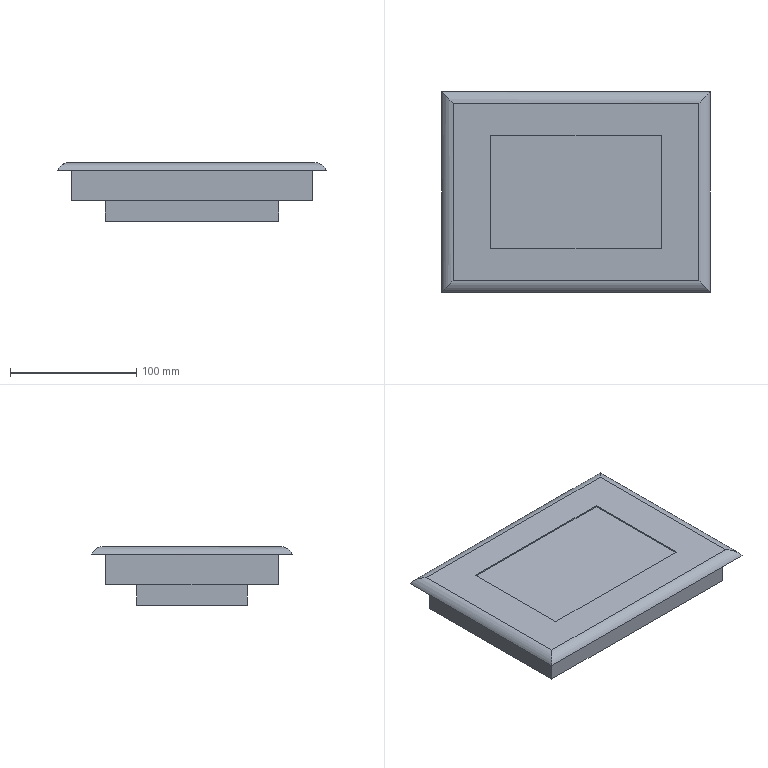Part | STEP file | 7-inch Weintek touch screen TH765-N[7-inch Weintek touch screen TH765-N]_7-inch Weintek touch screen TH765-N | 1 solid | 21 faces | box 213 x 159 x 46.5 mm | volume 1006657 mm3 | plane 17 | cylinder 4 | commonest cylinder face diameters 20 x4
STEP:
#1=CARTESIAN_POINT('',(97.335,-70.335,6.));
#2=VERTEX_POINT('',#1);
#3=CARTESIAN_POINT('',(-97.335,-70.335,6.));
#4=VERTEX_POINT('',#3);
#5=CARTESIAN_POINT('',(0.,-70.335,6.));
#6=DIRECTION('',(-1.,0.,0.));
#7=VECTOR('',#6,1000.);
#8=LINE('',#5,#7);
#9=EDGE_CURVE('',#2,#4,#8,.T.);
#10=ORIENTED_EDGE('',*,*,#9,.F.);
#11=CARTESIAN_POINT('',(97.335,70.335,6.));
#12=VERTEX_POINT('',#11);
#13=CARTESIAN_POINT('',(97.335,0.,6.));
#14=DIRECTION('',(0.,-1.,0.));
#15=VECTOR('',#14,1000.);
#16=LINE('',#13,#15);
#17=EDGE_CURVE('',#12,#2,#16,.T.);
#18=ORIENTED_EDGE('',*,*,#17,.F.);
#19=CARTESIAN_POINT('',(-97.335,70.335,6.));
#20=VERTEX_POINT('',#19);
#21=CARTESIAN_POINT('',(0.,70.335,6.));
#22=DIRECTION('',(1.,0.,0.));
#23=VECTOR('',#22,1000.);
#24=LINE('',#21,#23);
#25=EDGE_CURVE('',#20,#12,#24,.T.);
#26=ORIENTED_EDGE('',*,*,#25,.F.);
#27=CARTESIAN_POINT('',(-97.335,0.,6.));
#28=DIRECTION('',(0.,1.,0.));
#29=VECTOR('',#28,1000.);
#30=LINE('',#27,#29);
#31=EDGE_CURVE('',#4,#20,#30,.T.);
#32=ORIENTED_EDGE('',*,*,#31,.F.);
#33=EDGE_LOOP('',(#10,#18,#26,#32));
#34=FACE_OUTER_BOUND('',#33,.T.);
#35=CARTESIAN_POINT('',(67.5,-45.,6.));
#36=VERTEX_POINT('',#35);
#37=CARTESIAN_POINT('',(67.5,45.,6.));
#38=VERTEX_POINT('',#37);
#39=CARTESIAN_POINT('',(67.5,0.,6.));
#40=DIRECTION('',(0.,1.,0.));
#41=VECTOR('',#40,1000.);
#42=LINE('',#39,#41);
#43=EDGE_CURVE('',#36,#38,#42,.T.);
#44=ORIENTED_EDGE('',*,*,#43,.F.);
#45=CARTESIAN_POINT('',(-67.5,-45.,6.));
#46=VERTEX_POINT('',#45);
#47=CARTESIAN_POINT('',(0.,-45.,6.));
#48=DIRECTION('',(1.,0.,0.));
#49=VECTOR('',#48,1000.);
#50=LINE('',#47,#49);
#51=EDGE_CURVE('',#46,#36,#50,.T.);
#52=ORIENTED_EDGE('',*,*,#51,.F.);
#53=CARTESIAN_POINT('',(-67.5,45.,6.));
#54=VERTEX_POINT('',#53);
#55=CARTESIAN_POINT('',(-67.5,0.,6.));
#56=DIRECTION('',(0.,-1.,0.));
#57=VECTOR('',#56,1000.);
#58=LINE('',#55,#57);
#59=EDGE_CURVE('',#54,#46,#58,.T.);
#60=ORIENTED_EDGE('',*,*,#59,.F.);
#61=CARTESIAN_POINT('',(0.,45.,6.));
#62=DIRECTION('',(-1.,0.,0.));
#63=VECTOR('',#62,1000.);
#64=LINE('',#61,#63);
#65=EDGE_CURVE('',#38,#54,#64,.T.);
#66=ORIENTED_EDGE('',*,*,#65,.F.);
#67=EDGE_LOOP('',(#44,#52,#60,#66));
#68=FACE_BOUND('',#67,.T.);
#69=CARTESIAN_POINT('',(0.,0.,6.));
#70=DIRECTION('',(0.,0.,-1.));
#71=DIRECTION('',(-1.,0.,0.));
#72=AXIS2_PLACEMENT_3D('',#69,#70,#71);
#73=PLANE('',#72);
#74=ADVANCED_FACE('',(#34,#68),#73,.F.);
#75=CARTESIAN_POINT('',(-106.5,-79.5,0.));
#76=VERTEX_POINT('',#75);
#77=CARTESIAN_POINT('',(-106.5,-79.5,0.));
#78=CARTESIAN_POINT('',(-104.861,-77.861,3.756));
#79=CARTESIAN_POINT('',(-101.433,-74.433,6.));
#80=CARTESIAN_POINT('',(-97.335,-70.335,6.));
#81=(BOUNDED_CURVE()B_SPLINE_CURVE(3,(#77,#78,#79,#80),.UNSPECIFIED.,.F.,.F.)B_SPLINE_CURVE_WITH_KNOTS((4,4),(3.553,4.712),.UNSPECIFIED.)CURVE()GEOMETRIC_REPRESENTATION_ITEM()RATIONAL_B_SPLINE_CURVE((1.,0.8911,0.8911,1.))REPRESENTATION_ITEM(''));
#82=EDGE_CURVE('',#76,#4,#81,.T.);
#83=ORIENTED_EDGE('',*,*,#82,.T.);
#84=ORIENTED_EDGE('',*,*,#31,.T.);
#85=CARTESIAN_POINT('',(-106.5,79.5,0.));
#86=VERTEX_POINT('',#85);
#87=CARTESIAN_POINT('',(-97.335,70.335,6.));
#88=CARTESIAN_POINT('',(-101.433,74.433,6.));
#89=CARTESIAN_POINT('',(-104.861,77.861,3.756));
#90=CARTESIAN_POINT('',(-106.5,79.5,0.));
#91=(BOUNDED_CURVE()B_SPLINE_CURVE(3,(#87,#88,#89,#90),.UNSPECIFIED.,.F.,.F.)B_SPLINE_CURVE_WITH_KNOTS((4,4),(4.712,5.872),.UNSPECIFIED.)CURVE()GEOMETRIC_REPRESENTATION_ITEM()RATIONAL_B_SPLINE_CURVE((1.,0.8911,0.8911,1.))REPRESENTATION_ITEM(''));
#92=EDGE_CURVE('',#20,#86,#91,.T.);
#93=ORIENTED_EDGE('',*,*,#92,.T.);
#94=CARTESIAN_POINT('',(-106.5,-79.5,0.));
#95=DIRECTION('',(0.,-1.,0.));
#96=VECTOR('',#95,1000.);
#97=LINE('',#94,#96);
#98=EDGE_CURVE('',#86,#76,#97,.T.);
#99=ORIENTED_EDGE('',*,*,#98,.T.);
#100=EDGE_LOOP('',(#83,#84,#93,#99));
#101=FACE_OUTER_BOUND('',#100,.T.);
#102=CARTESIAN_POINT('',(-97.335,-79.5,-4.));
#103=DIRECTION('',(0.,1.,0.));
#104=DIRECTION('',(0.,0.,1.));
#105=AXIS2_PLACEMENT_3D('',#102,#103,#104);
#106=CYLINDRICAL_SURFACE('',#105,10.);
#107=ADVANCED_FACE('',(#101),#106,.T.);
#108=CARTESIAN_POINT('',(106.5,-79.5,0.));
#109=VERTEX_POINT('',#108);
#110=CARTESIAN_POINT('',(106.5,-79.5,0.));
#111=CARTESIAN_POINT('',(104.861,-77.861,3.756));
#112=CARTESIAN_POINT('',(101.433,-74.433,6.));
#113=CARTESIAN_POINT('',(97.335,-70.335,6.));
#114=(BOUNDED_CURVE()B_SPLINE_CURVE(3,(#110,#111,#112,#113),.UNSPECIFIED.,.F.,.F.)B_SPLINE_CURVE_WITH_KNOTS((4,4),(3.553,4.712),.UNSPECIFIED.)CURVE()GEOMETRIC_REPRESENTATION_ITEM()RATIONAL_B_SPLINE_CURVE((1.,0.8911,0.8911,1.))REPRESENTATION_ITEM(''));
#115=EDGE_CURVE('',#109,#2,#114,.T.);
#116=ORIENTED_EDGE('',*,*,#115,.T.);
#117=ORIENTED_EDGE('',*,*,#9,.T.);
#118=ORIENTED_EDGE('',*,*,#82,.F.);
#119=CARTESIAN_POINT('',(-106.5,-79.5,0.));
#120=DIRECTION('',(1.,0.,0.));
#121=VECTOR('',#120,1000.);
#122=LINE('',#119,#121);
#123=EDGE_CURVE('',#76,#109,#122,.T.);
#124=ORIENTED_EDGE('',*,*,#123,.T.);
#125=EDGE_LOOP('',(#116,#117,#118,#124));
#126=FACE_OUTER_BOUND('',#125,.T.);
#127=CARTESIAN_POINT('',(-106.5,-70.335,-4.));
#128=DIRECTION('',(-1.,0.,0.));
#129=DIRECTION('',(0.,0.,1.));
#130=AXIS2_PLACEMENT_3D('',#127,#128,#129);
#131=CYLINDRICAL_SURFACE('',#130,10.);
#132=ADVANCED_FACE('',(#126),#131,.T.);
#133=ORIENTED_EDGE('',*,*,#115,.F.);
#134=CARTESIAN_POINT('',(106.5,79.5,0.));
#135=VERTEX_POINT('',#134);
#136=CARTESIAN_POINT('',(106.5,-79.5,0.));
#137=DIRECTION('',(0.,1.,0.));
#138=VECTOR('',#137,1000.);
#139=LINE('',#136,#138);
#140=EDGE_CURVE('',#109,#135,#139,.T.);
#141=ORIENTED_EDGE('',*,*,#140,.T.);
#142=CARTESIAN_POINT('',(106.5,79.5,0.));
#143=CARTESIAN_POINT('',(104.861,77.861,3.756));
#144=CARTESIAN_POINT('',(101.433,74.433,6.));
#145=CARTESIAN_POINT('',(97.335,70.335,6.));
#146=(BOUNDED_CURVE()B_SPLINE_CURVE(3,(#142,#143,#144,#145),.UNSPECIFIED.,.F.,.F.)B_SPLINE_CURVE_WITH_KNOTS((4,4),(3.553,4.712),.UNSPECIFIED.)CURVE()GEOMETRIC_REPRESENTATION_ITEM()RATIONAL_B_SPLINE_CURVE((1.,0.8911,0.8911,1.))REPRESENTATION_ITEM(''));
#147=EDGE_CURVE('',#135,#12,#146,.T.);
#148=ORIENTED_EDGE('',*,*,#147,.T.);
#149=ORIENTED_EDGE('',*,*,#17,.T.);
#150=EDGE_LOOP('',(#133,#141,#148,#149));
#151=FACE_OUTER_BOUND('',#150,.T.);
#152=CARTESIAN_POINT('',(97.335,-79.5,-4.));
#153=DIRECTION('',(0.,-1.,0.));
#154=DIRECTION('',(0.,0.,-1.));
#155=AXIS2_PLACEMENT_3D('',#152,#153,#154);
#156=CYLINDRICAL_SURFACE('',#155,10.);
#157=ADVANCED_FACE('',(#151),#156,.T.);
#158=ORIENTED_EDGE('',*,*,#92,.F.);
#159=ORIENTED_EDGE('',*,*,#25,.T.);
#160=ORIENTED_EDGE('',*,*,#147,.F.);
#161=CARTESIAN_POINT('',(-106.5,79.5,0.));
#162=DIRECTION('',(-1.,0.,0.));
#163=VECTOR('',#162,1000.);
#164=LINE('',#161,#163);
#165=EDGE_CURVE('',#135,#86,#164,.T.);
#166=ORIENTED_EDGE('',*,*,#165,.T.);
#167=EDGE_LOOP('',(#158,#159,#160,#166));
#168=FACE_OUTER_BOUND('',#167,.T.);
#169=CARTESIAN_POINT('',(-106.5,70.335,-4.));
#170=DIRECTION('',(1.,0.,0.));
#171=DIRECTION('',(0.,0.,-1.));
#172=AXIS2_PLACEMENT_3D('',#169,#170,#171);
#173=CYLINDRICAL_SURFACE('',#172,10.);
#174=ADVANCED_FACE('',(#168),#173,.T.);
#175=CARTESIAN_POINT('',(-67.5,45.,5.));
#176=VERTEX_POINT('',#175);
#177=CARTESIAN_POINT('',(-67.5,45.,5.));
#178=DIRECTION('',(0.,0.,1.));
#179=VECTOR('',#178,1000.);
#180=LINE('',#177,#179);
#181=EDGE_CURVE('',#176,#54,#180,.T.);
#182=ORIENTED_EDGE('',*,*,#181,.F.);
#183=CARTESIAN_POINT('',(67.5,45.,5.));
#184=VERTEX_POINT('',#183);
#185=CARTESIAN_POINT('',(-67.5,45.,5.));
#186=DIRECTION('',(-1.,0.,0.));
#187=VECTOR('',#186,1000.);
#188=LINE('',#185,#187);
#189=EDGE_CURVE('',#184,#176,#188,.T.);
#190=ORIENTED_EDGE('',*,*,#189,.F.);
#191=CARTESIAN_POINT('',(67.5,45.,5.));
#192=DIRECTION('',(0.,0.,-1.));
#193=VECTOR('',#192,1000.);
#194=LINE('',#191,#193);
#195=EDGE_CURVE('',#38,#184,#194,.T.);
#196=ORIENTED_EDGE('',*,*,#195,.F.);
#197=ORIENTED_EDGE('',*,*,#65,.T.);
#198=EDGE_LOOP('',(#182,#190,#196,#197));
#199=FACE_OUTER_BOUND('',#198,.T.);
#200=CARTESIAN_POINT('',(-67.5,45.,5.));
#201=DIRECTION('',(0.,1.,0.));
#202=DIRECTION('',(0.,0.,1.));
#203=AXIS2_PLACEMENT_3D('',#200,#201,#202);
#204=PLANE('',#203);
#205=ADVANCED_FACE('',(#199),#204,.F.);
#206=ORIENTED_EDGE('',*,*,#195,.T.);
#207=CARTESIAN_POINT('',(67.5,-45.,5.));
#208=VERTEX_POINT('',#207);
#209=CARTESIAN_POINT('',(67.5,-45.,5.));
#210=DIRECTION('',(0.,1.,0.));
#211=VECTOR('',#210,1000.);
#212=LINE('',#209,#211);
#213=EDGE_CURVE('',#208,#184,#212,.T.);
#214=ORIENTED_EDGE('',*,*,#213,.F.);
#215=CARTESIAN_POINT('',(67.5,-45.,5.));
#216=DIRECTION('',(0.,0.,-1.));
#217=VECTOR('',#216,1000.);
#218=LINE('',#215,#217);
#219=EDGE_CURVE('',#36,#208,#218,.T.);
#220=ORIENTED_EDGE('',*,*,#219,.F.);
#221=ORIENTED_EDGE('',*,*,#43,.T.);
#222=EDGE_LOOP('',(#206,#214,#220,#221));
#223=FACE_OUTER_BOUND('',#222,.T.);
#224=CARTESIAN_POINT('',(67.5,-45.,5.));
#225=DIRECTION('',(1.,0.,0.));
#226=DIRECTION('',(0.,0.,-1.));
#227=AXIS2_PLACEMENT_3D('',#224,#225,#226);
#228=PLANE('',#227);
#229=ADVANCED_FACE('',(#223),#228,.F.);
#230=ORIENTED_EDGE('',*,*,#219,.T.);
#231=CARTESIAN_POINT('',(-67.5,-45.,5.));
#232=VERTEX_POINT('',#231);
#233=CARTESIAN_POINT('',(-67.5,-45.,5.));
#234=DIRECTION('',(1.,0.,0.));
#235=VECTOR('',#234,1000.);
#236=LINE('',#233,#235);
#237=EDGE_CURVE('',#232,#208,#236,.T.);
#238=ORIENTED_EDGE('',*,*,#237,.F.);
#239=CARTESIAN_POINT('',(-67.5,-45.,5.));
#240=DIRECTION('',(0.,0.,-1.));
#241=VECTOR('',#240,1000.);
#242=LINE('',#239,#241);
#243=EDGE_CURVE('',#46,#232,#242,.T.);
#244=ORIENTED_EDGE('',*,*,#243,.F.);
#245=ORIENTED_EDGE('',*,*,#51,.T.);
#246=EDGE_LOOP('',(#230,#238,#244,#245));
#247=FACE_OUTER_BOUND('',#246,.T.);
#248=CARTESIAN_POINT('',(-67.5,-45.,5.));
#249=DIRECTION('',(0.,-1.,0.));
#250=DIRECTION('',(0.,0.,-1.));
#251=AXIS2_PLACEMENT_3D('',#248,#249,#250);
#252=PLANE('',#251);
#253=ADVANCED_FACE('',(#247),#252,.F.);
#254=ORIENTED_EDGE('',*,*,#243,.T.);
#255=CARTESIAN_POINT('',(-67.5,-45.,5.));
#256=DIRECTION('',(0.,-1.,0.));
#257=VECTOR('',#256,1000.);
#258=LINE('',#255,#257);
#259=EDGE_CURVE('',#176,#232,#258,.T.);
#260=ORIENTED_EDGE('',*,*,#259,.F.);
#261=ORIENTED_EDGE('',*,*,#181,.T.);
#262=ORIENTED_EDGE('',*,*,#59,.T.);
#263=EDGE_LOOP('',(#254,#260,#261,#262));
#264=FACE_OUTER_BOUND('',#263,.T.);
#265=CARTESIAN_POINT('',(-67.5,-45.,5.));
#266=DIRECTION('',(-1.,0.,0.));
#267=DIRECTION('',(0.,0.,1.));
#268=AXIS2_PLACEMENT_3D('',#265,#266,#267);
#269=PLANE('',#268);
#270=ADVANCED_FACE('',(#264),#269,.F.);
#271=CARTESIAN_POINT('',(-95.5,-68.5,0.));
#272=VERTEX_POINT('',#271);
#273=CARTESIAN_POINT('',(95.5,-68.5,0.));
#274=VERTEX_POINT('',#273);
#275=CARTESIAN_POINT('',(0.,-68.5,0.));
#276=DIRECTION('',(1.,0.,0.));
#277=VECTOR('',#276,1000.);
#278=LINE('',#275,#277);
#279=EDGE_CURVE('',#272,#274,#278,.T.);
#280=ORIENTED_EDGE('',*,*,#279,.T.);
#281=CARTESIAN_POINT('',(95.5,68.5,0.));
#282=VERTEX_POINT('',#281);
#283=CARTESIAN_POINT('',(95.5,0.,0.));
#284=DIRECTION('',(0.,1.,0.));
#285=VECTOR('',#284,1000.);
#286=LINE('',#283,#285);
#287=EDGE_CURVE('',#274,#282,#286,.T.);
#288=ORIENTED_EDGE('',*,*,#287,.T.);
#289=CARTESIAN_POINT('',(-95.5,68.5,0.));
#290=VERTEX_POINT('',#289);
#291=CARTESIAN_POINT('',(0.,68.5,0.));
#292=DIRECTION('',(-1.,0.,0.));
#293=VECTOR('',#292,1000.);
#294=LINE('',#291,#293);
#295=EDGE_CURVE('',#282,#290,#294,.T.);
#296=ORIENTED_EDGE('',*,*,#295,.T.);
#297=CARTESIAN_POINT('',(-95.5,0.,0.));
#298=DIRECTION('',(0.,-1.,0.));
#299=VECTOR('',#298,1000.);
#300=LINE('',#297,#299);
#301=EDGE_CURVE('',#290,#272,#300,.T.);
#302=ORIENTED_EDGE('',*,*,#301,.T.);
#303=EDGE_LOOP('',(#280,#288,#296,#302));
#304=FACE_BOUND('',#303,.T.);
#305=ORIENTED_EDGE('',*,*,#98,.F.);
#306=ORIENTED_EDGE('',*,*,#165,.F.);
#307=ORIENTED_EDGE('',*,*,#140,.F.);
#308=ORIENTED_EDGE('',*,*,#123,.F.);
#309=EDGE_LOOP('',(#305,#306,#307,#308));
#310=FACE_OUTER_BOUND('',#309,.T.);
#311=CARTESIAN_POINT('',(0.,0.,0.));
#312=DIRECTION('',(0.,0.,-1.));
#313=DIRECTION('',(-1.,0.,0.));
#314=AXIS2_PLACEMENT_3D('',#311,#312,#313);
#315=PLANE('',#314);
#316=ADVANCED_FACE('',(#304,#310),#315,.T.);
#317=ORIENTED_EDGE('',*,*,#189,.T.);
#318=ORIENTED_EDGE('',*,*,#259,.T.);
#319=ORIENTED_EDGE('',*,*,#237,.T.);
#320=ORIENTED_EDGE('',*,*,#213,.T.);
#321=EDGE_LOOP('',(#317,#318,#319,#320));
#322=FACE_OUTER_BOUND('',#321,.T.);
#323=CARTESIAN_POINT('',(0.,0.,5.));
#324=DIRECTION('',(0.,0.,-1.));
#325=DIRECTION('',(-1.,0.,0.));
#326=AXIS2_PLACEMENT_3D('',#323,#324,#325);
#327=PLANE('',#326);
#328=ADVANCED_FACE('',(#322),#327,.F.);
#329=CARTESIAN_POINT('',(95.5,-68.5,-24.));
#330=VERTEX_POINT('',#329);
#331=CARTESIAN_POINT('',(95.5,-68.5,-24.));
#332=DIRECTION('',(0.,0.,1.));
#333=VECTOR('',#332,1000.);
#334=LINE('',#331,#333);
#335=EDGE_CURVE('',#330,#274,#334,.T.);
#336=ORIENTED_EDGE('',*,*,#335,.F.);
#337=CARTESIAN_POINT('',(95.5,68.5,-24.));
#338=VERTEX_POINT('',#337);
#339=CARTESIAN_POINT('',(95.5,-68.5,-24.));
#340=DIRECTION('',(0.,-1.,0.));
#341=VECTOR('',#340,1000.);
#342=LINE('',#339,#341);
#343=EDGE_CURVE('',#338,#330,#342,.T.);
#344=ORIENTED_EDGE('',*,*,#343,.F.);
#345=CARTESIAN_POINT('',(95.5,68.5,-24.));
#346=DIRECTION('',(0.,0.,-1.));
#347=VECTOR('',#346,1000.);
#348=LINE('',#345,#347);
#349=EDGE_CURVE('',#282,#338,#348,.T.);
#350=ORIENTED_EDGE('',*,*,#349,.F.);
#351=ORIENTED_EDGE('',*,*,#287,.F.);
#352=EDGE_LOOP('',(#336,#344,#350,#351));
#353=FACE_OUTER_BOUND('',#352,.T.);
#354=CARTESIAN_POINT('',(95.5,-68.5,-24.));
#355=DIRECTION('',(-1.,0.,0.));
#356=DIRECTION('',(0.,0.,1.));
#357=AXIS2_PLACEMENT_3D('',#354,#355,#356);
#358=PLANE('',#357);
#359=ADVANCED_FACE('',(#353),#358,.F.);
#360=CARTESIAN_POINT('',(-95.5,-68.5,-24.));
#361=VERTEX_POINT('',#360);
#362=CARTESIAN_POINT('',(-95.5,-68.5,-24.));
#363=DIRECTION('',(0.,0.,1.));
#364=VECTOR('',#363,1000.);
#365=LINE('',#362,#364);
#366=EDGE_CURVE('',#361,#272,#365,.T.);
#367=ORIENTED_EDGE('',*,*,#366,.F.);
#368=CARTESIAN_POINT('',(95.5,-68.5,-24.));
#369=DIRECTION('',(-1.,0.,0.));
#370=VECTOR('',#369,1000.);
#371=LINE('',#368,#370);
#372=EDGE_CURVE('',#330,#361,#371,.T.);
#373=ORIENTED_EDGE('',*,*,#372,.F.);
#374=ORIENTED_EDGE('',*,*,#335,.T.);
#375=ORIENTED_EDGE('',*,*,#279,.F.);
#376=EDGE_LOOP('',(#367,#373,#374,#375));
#377=FACE_OUTER_BOUND('',#376,.T.);
#378=CARTESIAN_POINT('',(95.5,-68.5,-24.));
#379=DIRECTION('',(0.,1.,0.));
#380=DIRECTION('',(0.,0.,1.));
#381=AXIS2_PLACEMENT_3D('',#378,#379,#380);
#382=PLANE('',#381);
#383=ADVANCED_FACE('',(#377),#382,.F.);
#384=CARTESIAN_POINT('',(-95.5,68.5,-24.));
#385=VERTEX_POINT('',#384);
#386=CARTESIAN_POINT('',(-95.5,68.5,-24.));
#387=DIRECTION('',(0.,0.,1.));
#388=VECTOR('',#387,1000.);
#389=LINE('',#386,#388);
#390=EDGE_CURVE('',#385,#290,#389,.T.);
#391=ORIENTED_EDGE('',*,*,#390,.F.);
#392=CARTESIAN_POINT('',(-95.5,-68.5,-24.));
#393=DIRECTION('',(0.,1.,0.));
#394=VECTOR('',#393,1000.);
#395=LINE('',#392,#394);
#396=EDGE_CURVE('',#361,#385,#395,.T.);
#397=ORIENTED_EDGE('',*,*,#396,.F.);
#398=ORIENTED_EDGE('',*,*,#366,.T.);
#399=ORIENTED_EDGE('',*,*,#301,.F.);
#400=EDGE_LOOP('',(#391,#397,#398,#399));
#401=FACE_OUTER_BOUND('',#400,.T.);
#402=CARTESIAN_POINT('',(-95.5,-68.5,-24.));
#403=DIRECTION('',(1.,0.,0.));
#404=DIRECTION('',(0.,0.,-1.));
#405=AXIS2_PLACEMENT_3D('',#402,#403,#404);
#406=PLANE('',#405);
#407=ADVANCED_FACE('',(#401),#406,.F.);
#408=ORIENTED_EDGE('',*,*,#349,.T.);
#409=CARTESIAN_POINT('',(95.5,68.5,-24.));
#410=DIRECTION('',(1.,0.,0.));
#411=VECTOR('',#410,1000.);
#412=LINE('',#409,#411);
#413=EDGE_CURVE('',#385,#338,#412,.T.);
#414=ORIENTED_EDGE('',*,*,#413,.F.);
#415=ORIENTED_EDGE('',*,*,#390,.T.);
#416=ORIENTED_EDGE('',*,*,#295,.F.);
#417=EDGE_LOOP('',(#408,#414,#415,#416));
#418=FACE_OUTER_BOUND('',#417,.T.);
#419=CARTESIAN_POINT('',(95.5,68.5,-24.));
#420=DIRECTION('',(0.,-1.,0.));
#421=DIRECTION('',(0.,0.,-1.));
#422=AXIS2_PLACEMENT_3D('',#419,#420,#421);
#423=PLANE('',#422);
#424=ADVANCED_FACE('',(#418),#423,.F.);
#425=CARTESIAN_POINT('',(68.782,-43.783,-24.));
#426=VERTEX_POINT('',#425);
#427=CARTESIAN_POINT('',(-68.782,-43.783,-24.));
#428=VERTEX_POINT('',#427);
#429=CARTESIAN_POINT('',(0.,-43.783,-24.));
#430=DIRECTION('',(-1.,0.,0.));
#431=VECTOR('',#430,1000.);
#432=LINE('',#429,#431);
#433=EDGE_CURVE('',#426,#428,#432,.T.);
#434=ORIENTED_EDGE('',*,*,#433,.F.);
#435=CARTESIAN_POINT('',(68.782,43.783,-24.));
#436=VERTEX_POINT('',#435);
#437=CARTESIAN_POINT('',(68.782,0.,-24.));
#438=DIRECTION('',(0.,-1.,0.));
#439=VECTOR('',#438,1000.);
#440=LINE('',#437,#439);
#441=EDGE_CURVE('',#436,#426,#440,.T.);
#442=ORIENTED_EDGE('',*,*,#441,.F.);
#443=CARTESIAN_POINT('',(-68.782,43.783,-24.));
#444=VERTEX_POINT('',#443);
#445=CARTESIAN_POINT('',(0.,43.783,-24.));
#446=DIRECTION('',(1.,0.,0.));
#447=VECTOR('',#446,1000.);
#448=LINE('',#445,#447);
#449=EDGE_CURVE('',#444,#436,#448,.T.);
#450=ORIENTED_EDGE('',*,*,#449,.F.);
#451=CARTESIAN_POINT('',(-68.782,0.,-24.));
#452=DIRECTION('',(0.,1.,0.));
#453=VECTOR('',#452,1000.);
#454=LINE('',#451,#453);
#455=EDGE_CURVE('',#428,#444,#454,.T.);
#456=ORIENTED_EDGE('',*,*,#455,.F.);
#457=EDGE_LOOP('',(#434,#442,#450,#456));
#458=FACE_BOUND('',#457,.T.);
#459=ORIENTED_EDGE('',*,*,#413,.T.);
#460=ORIENTED_EDGE('',*,*,#343,.T.);
#461=ORIENTED_EDGE('',*,*,#372,.T.);
#462=ORIENTED_EDGE('',*,*,#396,.T.);
#463=EDGE_LOOP('',(#459,#460,#461,#462));
#464=FACE_OUTER_BOUND('',#463,.T.);
#465=CARTESIAN_POINT('',(0.,0.,-24.));
#466=DIRECTION('',(0.,0.,1.));
#467=DIRECTION('',(1.,0.,0.));
#468=AXIS2_PLACEMENT_3D('',#465,#466,#467);
#469=PLANE('',#468);
#470=ADVANCED_FACE('',(#458,#464),#469,.F.);
#471=CARTESIAN_POINT('',(-68.782,43.783,-40.5));
#472=VERTEX_POINT('',#471);
#473=CARTESIAN_POINT('',(-68.782,43.783,-40.5));
#474=DIRECTION('',(0.,0.,1.));
#475=VECTOR('',#474,1000.);
#476=LINE('',#473,#475);
#477=EDGE_CURVE('',#472,#444,#476,.T.);
#478=ORIENTED_EDGE('',*,*,#477,.F.);
#479=CARTESIAN_POINT('',(-68.782,-43.783,-40.5));
#480=VERTEX_POINT('',#479);
#481=CARTESIAN_POINT('',(-68.782,-43.783,-40.5));
#482=DIRECTION('',(0.,1.,0.));
#483=VECTOR('',#482,1000.);
#484=LINE('',#481,#483);
#485=EDGE_CURVE('',#480,#472,#484,.T.);
#486=ORIENTED_EDGE('',*,*,#485,.F.);
#487=CARTESIAN_POINT('',(-68.782,-43.783,-40.5));
#488=DIRECTION('',(0.,0.,-1.));
#489=VECTOR('',#488,1000.);
#490=LINE('',#487,#489);
#491=EDGE_CURVE('',#428,#480,#490,.T.);
#492=ORIENTED_EDGE('',*,*,#491,.F.);
#493=ORIENTED_EDGE('',*,*,#455,.T.);
#494=EDGE_LOOP('',(#478,#486,#492,#493));
#495=FACE_OUTER_BOUND('',#494,.T.);
#496=CARTESIAN_POINT('',(-68.782,-43.783,-40.5));
#497=DIRECTION('',(1.,0.,0.));
#498=DIRECTION('',(0.,0.,-1.));
#499=AXIS2_PLACEMENT_3D('',#496,#497,#498);
#500=PLANE('',#499);
#501=ADVANCED_FACE('',(#495),#500,.F.);
#502=ORIENTED_EDGE('',*,*,#491,.T.);
#503=CARTESIAN_POINT('',(68.782,-43.783,-40.5));
#504=VERTEX_POINT('',#503);
#505=CARTESIAN_POINT('',(68.782,-43.783,-40.5));
#506=DIRECTION('',(-1.,0.,0.));
#507=VECTOR('',#506,1000.);
#508=LINE('',#505,#507);
#509=EDGE_CURVE('',#504,#480,#508,.T.);
#510=ORIENTED_EDGE('',*,*,#509,.F.);
#511=CARTESIAN_POINT('',(68.782,-43.783,-40.5));
#512=DIRECTION('',(0.,0.,-1.));
#513=VECTOR('',#512,1000.);
#514=LINE('',#511,#513);
#515=EDGE_CURVE('',#426,#504,#514,.T.);
#516=ORIENTED_EDGE('',*,*,#515,.F.);
#517=ORIENTED_EDGE('',*,*,#433,.T.);
#518=EDGE_LOOP('',(#502,#510,#516,#517));
#519=FACE_OUTER_BOUND('',#518,.T.);
#520=CARTESIAN_POINT('',(68.782,-43.783,-40.5));
#521=DIRECTION('',(0.,1.,0.));
#522=DIRECTION('',(0.,0.,1.));
#523=AXIS2_PLACEMENT_3D('',#520,#521,#522);
#524=PLANE('',#523);
#525=ADVANCED_FACE('',(#519),#524,.F.);
#526=ORIENTED_EDGE('',*,*,#515,.T.);
#527=CARTESIAN_POINT('',(68.782,43.783,-40.5));
#528=VERTEX_POINT('',#527);
#529=CARTESIAN_POINT('',(68.782,-43.783,-40.5));
#530=DIRECTION('',(0.,-1.,0.));
#531=VECTOR('',#530,1000.);
#532=LINE('',#529,#531);
#533=EDGE_CURVE('',#528,#504,#532,.T.);
#534=ORIENTED_EDGE('',*,*,#533,.F.);
#535=CARTESIAN_POINT('',(68.782,43.783,-40.5));
#536=DIRECTION('',(0.,0.,-1.));
#537=VECTOR('',#536,1000.);
#538=LINE('',#535,#537);
#539=EDGE_CURVE('',#436,#528,#538,.T.);
#540=ORIENTED_EDGE('',*,*,#539,.F.);
#541=ORIENTED_EDGE('',*,*,#441,.T.);
#542=EDGE_LOOP('',(#526,#534,#540,#541));
#543=FACE_OUTER_BOUND('',#542,.T.);
#544=CARTESIAN_POINT('',(68.782,-43.783,-40.5));
#545=DIRECTION('',(-1.,0.,0.));
#546=DIRECTION('',(0.,0.,1.));
#547=AXIS2_PLACEMENT_3D('',#544,#545,#546);
#548=PLANE('',#547);
#549=ADVANCED_FACE('',(#543),#548,.F.);
#550=ORIENTED_EDGE('',*,*,#539,.T.);
#551=CARTESIAN_POINT('',(68.782,43.783,-40.5));
#552=DIRECTION('',(1.,0.,0.));
#553=VECTOR('',#552,1000.);
#554=LINE('',#551,#553);
#555=EDGE_CURVE('',#472,#528,#554,.T.);
#556=ORIENTED_EDGE('',*,*,#555,.F.);
#557=ORIENTED_EDGE('',*,*,#477,.T.);
#558=ORIENTED_EDGE('',*,*,#449,.T.);
#559=EDGE_LOOP('',(#550,#556,#557,#558));
#560=FACE_OUTER_BOUND('',#559,.T.);
#561=CARTESIAN_POINT('',(68.782,43.783,-40.5));
#562=DIRECTION('',(0.,-1.,0.));
#563=DIRECTION('',(0.,0.,-1.));
#564=AXIS2_PLACEMENT_3D('',#561,#562,#563);
#565=PLANE('',#564);
#566=ADVANCED_FACE('',(#560),#565,.F.);
#567=ORIENTED_EDGE('',*,*,#555,.T.);
#568=ORIENTED_EDGE('',*,*,#533,.T.);
#569=ORIENTED_EDGE('',*,*,#509,.T.);
#570=ORIENTED_EDGE('',*,*,#485,.T.);
#571=EDGE_LOOP('',(#567,#568,#569,#570));
#572=FACE_OUTER_BOUND('',#571,.T.);
#573=CARTESIAN_POINT('',(0.,0.,-40.5));
#574=DIRECTION('',(0.,0.,1.));
#575=DIRECTION('',(1.,0.,0.));
#576=AXIS2_PLACEMENT_3D('',#573,#574,#575);
#577=PLANE('',#576);
#578=ADVANCED_FACE('',(#572),#577,.F.);
#579=CLOSED_SHELL('',(#74,#107,#132,#157,#174,#205,#229,#253,#270,#316,#328,#359,#383,#407,#424,#470,#501,#525,#549,#566,#578));
#580=MANIFOLD_SOLID_BREP('',#579);
#581=CARTESIAN_POINT('',(0.,0.,0.));
#582=DIRECTION('',(0.,0.,1.));
#583=DIRECTION('',(1.,0.,0.));
#584=AXIS2_PLACEMENT_3D('',#581,#582,#583);
#585=(LENGTH_UNIT()NAMED_UNIT(*)SI_UNIT(.MILLI.,.METRE.));
#586=UNCERTAINTY_MEASURE_WITH_UNIT(LENGTH_MEASURE(0.00001),#585,'','');
#587=(NAMED_UNIT(*)PLANE_ANGLE_UNIT()SI_UNIT($,.RADIAN.));
#588=(NAMED_UNIT(*)SI_UNIT($,.STERADIAN.)SOLID_ANGLE_UNIT());
#589=(GEOMETRIC_REPRESENTATION_CONTEXT(3)GLOBAL_UNCERTAINTY_ASSIGNED_CONTEXT((#586))GLOBAL_UNIT_ASSIGNED_CONTEXT((#585,#587,#588))REPRESENTATION_CONTEXT('',''));
#590=ADVANCED_BREP_SHAPE_REPRESENTATION('',(#580,#584),#589);